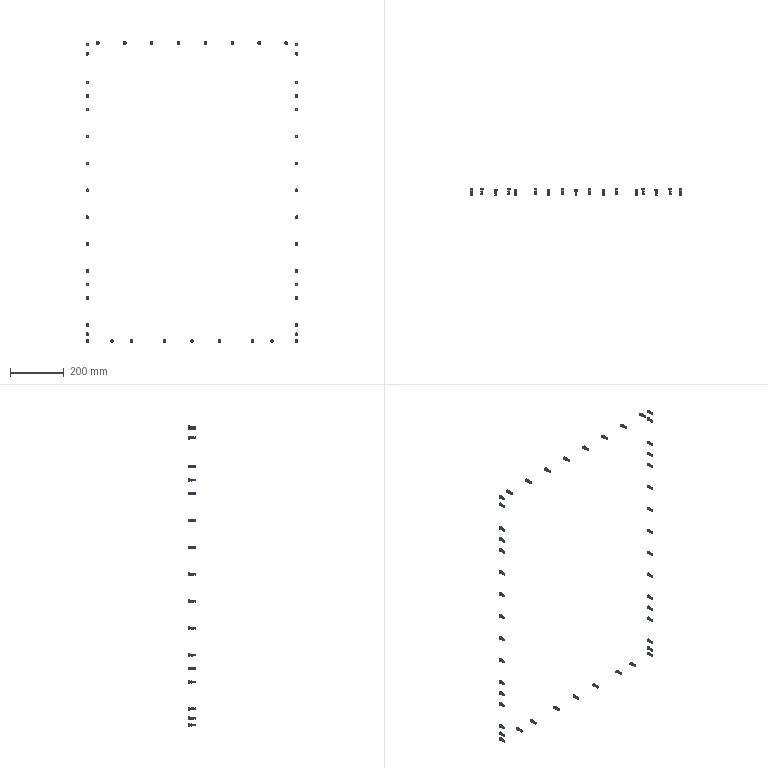Part | NX | features BREP 1 | 47 solids | 6110 faces | volume 31916 mm3 | spline 3572 | plane 1128 | cylinder 752 | torus 282 | sphere 282 | cone 94 | commonest cylinder face diameters 1 x329 5 x141 6.1 x94 6.9 x94 10 x94